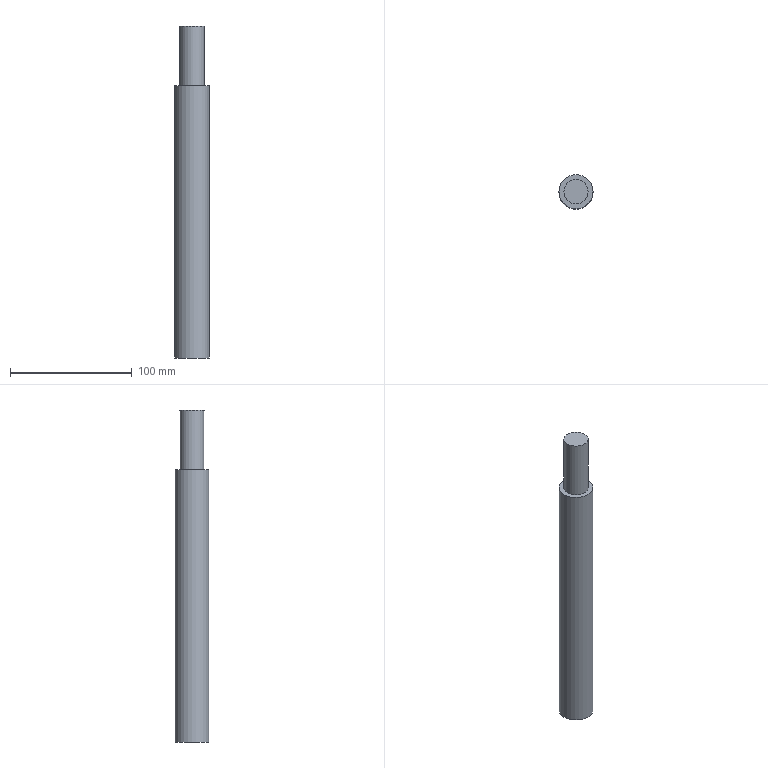Part | NX | features solid 2 | 1 solid | 5 faces | box 28 x 28 x 273 mm | volume 153322 mm3 | plane 3 | cylinder 2 | commonest cylinder face diameters 20 x1 28 x1
STEP:
#1=CARTESIAN_POINT('',(14.,-60.,-49.));
#2=VERTEX_POINT('',#1);
#3=CARTESIAN_POINT('',(0.,-60.,-49.));
#4=DIRECTION('',(0.,0.,1.));
#5=DIRECTION('',(1.,0.,0.));
#6=AXIS2_PLACEMENT_3D('',#3,#4,#5);
#7=CIRCLE('',#6,14.);
#8=EDGE_CURVE('',#2,#2,#7,.T.);
#9=ORIENTED_EDGE('',*,*,#8,.F.);
#10=EDGE_LOOP('',(#9));
#11=FACE_BOUND('',#10,.T.);
#12=CARTESIAN_POINT('',(14.,-60.,-273.));
#13=VERTEX_POINT('',#12);
#14=CARTESIAN_POINT('',(0.,-60.,-273.));
#15=DIRECTION('',(0.,0.,1.));
#16=DIRECTION('',(1.,0.,0.));
#17=AXIS2_PLACEMENT_3D('',#14,#15,#16);
#18=CIRCLE('',#17,14.);
#19=EDGE_CURVE('',#13,#13,#18,.T.);
#20=ORIENTED_EDGE('',*,*,#19,.T.);
#21=EDGE_LOOP('',(#20));
#22=FACE_BOUND('',#21,.T.);
#23=CARTESIAN_POINT('',(0.,-60.,-273.));
#24=DIRECTION('',(0.,0.,1.));
#25=DIRECTION('',(1.,0.,0.));
#26=AXIS2_PLACEMENT_3D('',#23,#24,#25);
#27=CYLINDRICAL_SURFACE('',#26,14.);
#28=ADVANCED_FACE('',(#11,#22),#27,.T.);
#29=ORIENTED_EDGE('',*,*,#19,.F.);
#30=EDGE_LOOP('',(#29));
#31=FACE_BOUND('',#30,.T.);
#32=CARTESIAN_POINT('',(0.,-60.,-273.));
#33=DIRECTION('',(0.,0.,1.));
#34=DIRECTION('',(1.,0.,0.));
#35=AXIS2_PLACEMENT_3D('',#32,#33,#34);
#36=PLANE('',#35);
#37=ADVANCED_FACE('',(#31),#36,.F.);
#38=ORIENTED_EDGE('',*,*,#8,.T.);
#39=EDGE_LOOP('',(#38));
#40=FACE_BOUND('',#39,.T.);
#41=CARTESIAN_POINT('',(-10.,-60.,-49.));
#42=VERTEX_POINT('',#41);
#43=CARTESIAN_POINT('',(0.,-60.,-49.));
#44=DIRECTION('',(0.,0.,-1.));
#45=DIRECTION('',(-1.,0.,0.));
#46=AXIS2_PLACEMENT_3D('',#43,#44,#45);
#47=CIRCLE('',#46,10.);
#48=EDGE_CURVE('',#42,#42,#47,.F.);
#49=ORIENTED_EDGE('',*,*,#48,.F.);
#50=EDGE_LOOP('',(#49));
#51=FACE_BOUND('',#50,.T.);
#52=CARTESIAN_POINT('',(0.,-60.,-49.));
#53=DIRECTION('',(0.,0.,-1.));
#54=DIRECTION('',(-1.,0.,0.));
#55=AXIS2_PLACEMENT_3D('',#52,#53,#54);
#56=PLANE('',#55);
#57=ADVANCED_FACE('',(#40,#51),#56,.F.);
#58=ORIENTED_EDGE('',*,*,#48,.T.);
#59=EDGE_LOOP('',(#58));
#60=FACE_BOUND('',#59,.T.);
#61=CARTESIAN_POINT('',(-10.,-60.,0.));
#62=VERTEX_POINT('',#61);
#63=CARTESIAN_POINT('',(0.,-60.,0.));
#64=DIRECTION('',(0.,0.,-1.));
#65=DIRECTION('',(-1.,0.,0.));
#66=AXIS2_PLACEMENT_3D('',#63,#64,#65);
#67=CIRCLE('',#66,10.);
#68=EDGE_CURVE('',#62,#62,#67,.F.);
#69=ORIENTED_EDGE('',*,*,#68,.F.);
#70=EDGE_LOOP('',(#69));
#71=FACE_BOUND('',#70,.T.);
#72=CARTESIAN_POINT('',(0.,-60.,0.));
#73=DIRECTION('',(0.,0.,-1.));
#74=DIRECTION('',(-1.,0.,0.));
#75=AXIS2_PLACEMENT_3D('',#72,#73,#74);
#76=CYLINDRICAL_SURFACE('',#75,10.);
#77=ADVANCED_FACE('',(#60,#71),#76,.T.);
#78=ORIENTED_EDGE('',*,*,#68,.T.);
#79=EDGE_LOOP('',(#78));
#80=FACE_BOUND('',#79,.T.);
#81=CARTESIAN_POINT('',(0.,-60.,0.));
#82=DIRECTION('',(0.,0.,1.));
#83=DIRECTION('',(1.,0.,0.));
#84=AXIS2_PLACEMENT_3D('',#81,#82,#83);
#85=PLANE('',#84);
#86=ADVANCED_FACE('',(#80),#85,.T.);
#87=CLOSED_SHELL('',(#28,#37,#57,#77,#86));
#88=MANIFOLD_SOLID_BREP('',#87);
#89=(LENGTH_UNIT()NAMED_UNIT(*)SI_UNIT(.MILLI.,.METRE.));
#90=UNCERTAINTY_MEASURE_WITH_UNIT(LENGTH_MEASURE(0.00001),#89,'','');
#91=(NAMED_UNIT(*)PLANE_ANGLE_UNIT()SI_UNIT($,.RADIAN.));
#92=(NAMED_UNIT(*)SI_UNIT($,.STERADIAN.)SOLID_ANGLE_UNIT());
#93=(GEOMETRIC_REPRESENTATION_CONTEXT(3)GLOBAL_UNCERTAINTY_ASSIGNED_CONTEXT((#90))GLOBAL_UNIT_ASSIGNED_CONTEXT((#89,#91,#92))REPRESENTATION_CONTEXT('',''));
#94=ADVANCED_BREP_SHAPE_REPRESENTATION('',(#88),#93);